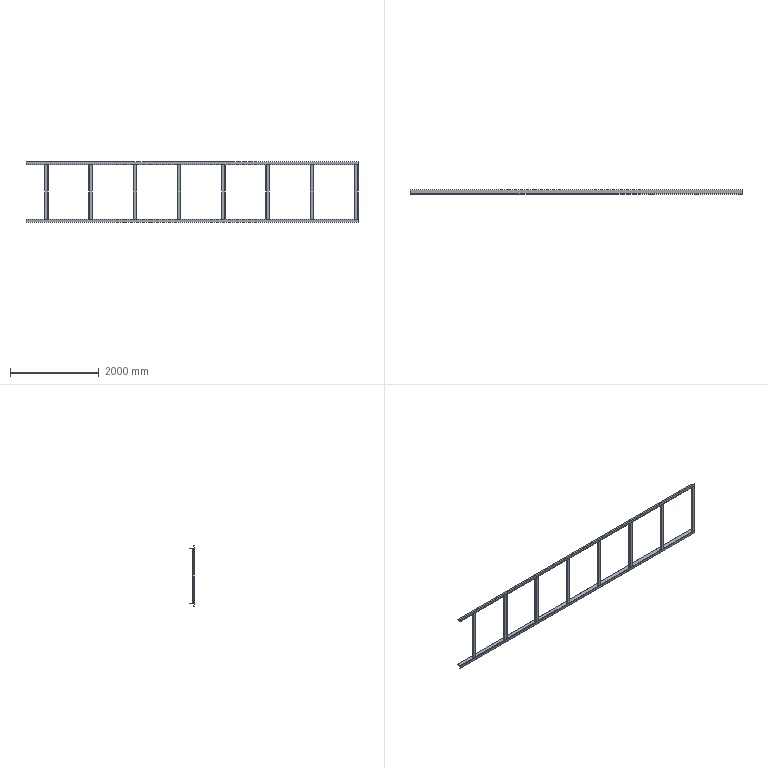Part | SolidWorks | features WeldMemberFeat 3, 3DProfileFeature 2, WeldmentFeature 1 | 10 solids | 166 faces | box 7500 x 100 x 1356 mm | volume 20928649 mm3 | plane 96 | cylinder 70 | commonest cylinder face diameters 6 x32 12 x32 4 x4 20 x2